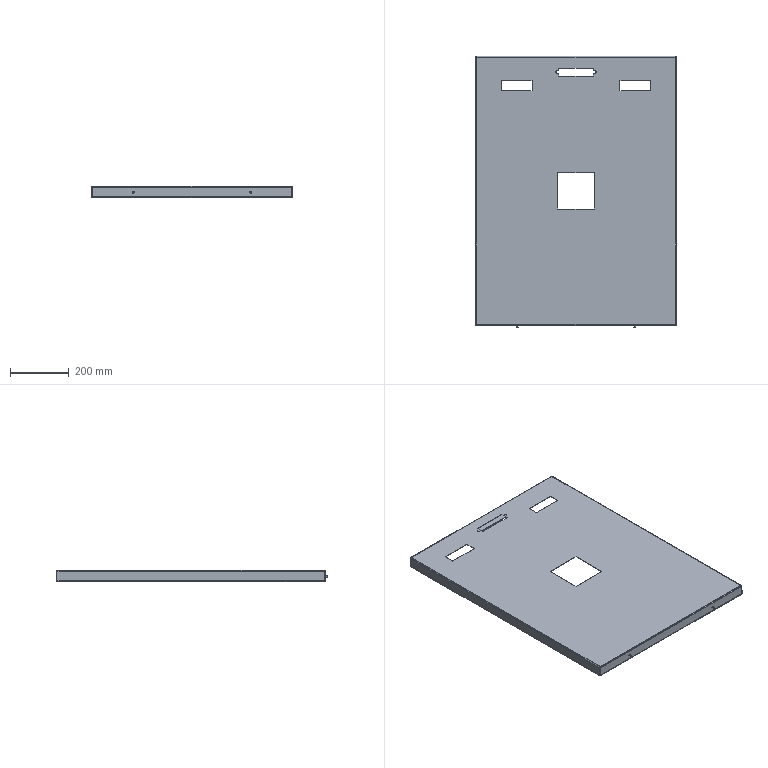Part | SolidWorks | features ICE 7, SMWeldBead 4, EdgeFlange 2, FlatPattern 1, SMBaseFlange 1, SheetMetal 1 | 1 solid | 149 faces | box 685 x 925 x 38 mm | volume 1176046 mm3 | plane 80 | spline 40 | cylinder 29 | commonest cylinder face diameters 4 x8 7 x8 6 x6 2 x4 9 x3